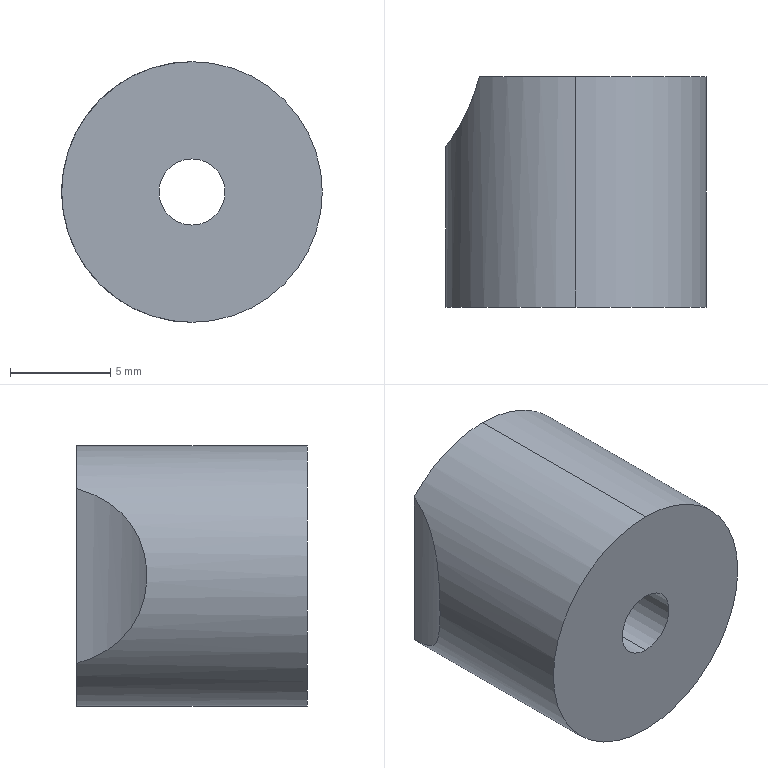Part | STEP file | BU-A15b | 1 solid | 7 faces | box 13 x 11.5 x 13 mm | volume 1411 mm3 | cylinder 5 | plane 2 | commonest cylinder face diameters 3.3 x2 13 x2 20 x1
STEP:
#1=CARTESIAN_POINT('',(0.,0.,0.));
#2=DIRECTION('',(0.,0.,1.));
#3=DIRECTION('',(1.,0.,0.));
#4=AXIS2_PLACEMENT_3D('',#1,#2,#3);
#5=CARTESIAN_POINT('',(0.,11.5,-1.65));
#6=VERTEX_POINT('',#5);
#7=CARTESIAN_POINT('',(0.,0.,-1.65));
#8=VERTEX_POINT('',#7);
#9=CARTESIAN_POINT('',(0.,0.,-1.65));
#10=DIRECTION('',(0.,-1.,0.));
#11=VECTOR('',#10,1.);
#12=LINE('',#9,#11);
#13=CARTESIAN_POINT('',(0.,0.,0.));
#14=DIRECTION('',(0.,-1.,0.));
#15=DIRECTION('',(0.,0.,-1.));
#16=AXIS2_PLACEMENT_3D('',#13,#14,#15);
#17=CYLINDRICAL_SURFACE('',#16,1.65);
#18=CARTESIAN_POINT('',(6.283,0.));
#19=DIRECTION('',(0.,1.));
#20=VECTOR('',#19,1.);
#21=LINE('',#18,#20);
#22=(GEOMETRIC_REPRESENTATION_CONTEXT(2)PARAMETRIC_REPRESENTATION_CONTEXT()REPRESENTATION_CONTEXT('',''));
#23=DEFINITIONAL_REPRESENTATION('',(#21),#22);
#24=PCURVE('',#17,#23);
#25=CARTESIAN_POINT('',(0.,0.,0.));
#26=DIRECTION('',(0.,-1.,0.));
#27=DIRECTION('',(0.,0.,-1.));
#28=AXIS2_PLACEMENT_3D('',#25,#26,#27);
#29=CYLINDRICAL_SURFACE('',#28,1.65);
#30=CARTESIAN_POINT('',(0.,0.));
#31=DIRECTION('',(0.,1.));
#32=VECTOR('',#31,1.);
#33=LINE('',#30,#32);
#34=(GEOMETRIC_REPRESENTATION_CONTEXT(2)PARAMETRIC_REPRESENTATION_CONTEXT()REPRESENTATION_CONTEXT('',''));
#35=DEFINITIONAL_REPRESENTATION('',(#33),#34);
#36=PCURVE('',#29,#35);
#37=SURFACE_CURVE('',#12,(#24,#36),.PCURVE_S1.);
#38=EDGE_CURVE('',#6,#8,#37,.T.);
#39=ORIENTED_EDGE('',*,*,#38,.T.);
#40=CARTESIAN_POINT('',(0.,0.,1.65));
#41=VERTEX_POINT('',#40);
#42=CARTESIAN_POINT('',(0.,0.,0.));
#43=DIRECTION('',(0.,-1.,0.));
#44=DIRECTION('',(0.,0.,-1.));
#45=AXIS2_PLACEMENT_3D('',#42,#43,#44);
#46=CIRCLE('',#45,1.65);
#47=CARTESIAN_POINT('',(0.,0.));
#48=DIRECTION('',(1.,0.));
#49=VECTOR('',#48,1.);
#50=LINE('',#47,#49);
#51=(GEOMETRIC_REPRESENTATION_CONTEXT(2)PARAMETRIC_REPRESENTATION_CONTEXT()REPRESENTATION_CONTEXT('',''));
#52=DEFINITIONAL_REPRESENTATION('',(#50),#51);
#53=PCURVE('',#17,#52);
#54=CARTESIAN_POINT('',(0.,0.,0.));
#55=DIRECTION('',(0.,1.,0.));
#56=DIRECTION('',(0.,0.,1.));
#57=AXIS2_PLACEMENT_3D('',#54,#55,#56);
#58=PLANE('',#57);
#59=CARTESIAN_POINT('',(-1.65,0.));
#60=CARTESIAN_POINT('',(-1.65,2.858));
#61=CARTESIAN_POINT('',(0.825,1.429));
#62=CARTESIAN_POINT('',(3.3,0.));
#63=CARTESIAN_POINT('',(0.825,-1.429));
#64=CARTESIAN_POINT('',(-1.65,-2.858));
#65=CARTESIAN_POINT('',(-1.65,0.));
#66=(BOUNDED_CURVE()B_SPLINE_CURVE(2,(#59,#60,#61,#62,#63,#64,#65),.UNSPECIFIED.,.T.,.F.)B_SPLINE_CURVE_WITH_KNOTS((1,2,2,2,2,1),(-2.094,0.,2.094,4.189,6.283,8.378),.UNSPECIFIED.)CURVE()GEOMETRIC_REPRESENTATION_ITEM()RATIONAL_B_SPLINE_CURVE((1.,0.5,1.,0.5,1.,0.5,1.))REPRESENTATION_ITEM(''));
#67=(GEOMETRIC_REPRESENTATION_CONTEXT(2)PARAMETRIC_REPRESENTATION_CONTEXT()REPRESENTATION_CONTEXT('',''));
#68=DEFINITIONAL_REPRESENTATION('',(#66),#67);
#69=PCURVE('',#58,#68);
#70=SURFACE_CURVE('',#46,(#53,#69),.PCURVE_S1.);
#71=EDGE_CURVE('',#41,#8,#70,.T.);
#72=ORIENTED_EDGE('',*,*,#71,.F.);
#73=CARTESIAN_POINT('',(0.,11.5,1.65));
#74=VERTEX_POINT('',#73);
#75=CARTESIAN_POINT('',(0.,0.,1.65));
#76=DIRECTION('',(0.,-1.,0.));
#77=VECTOR('',#76,1.);
#78=LINE('',#75,#77);
#79=CARTESIAN_POINT('',(3.142,0.));
#80=DIRECTION('',(0.,1.));
#81=VECTOR('',#80,1.);
#82=LINE('',#79,#81);
#83=(GEOMETRIC_REPRESENTATION_CONTEXT(2)PARAMETRIC_REPRESENTATION_CONTEXT()REPRESENTATION_CONTEXT('',''));
#84=DEFINITIONAL_REPRESENTATION('',(#82),#83);
#85=PCURVE('',#17,#84);
#86=CARTESIAN_POINT('',(3.142,0.));
#87=DIRECTION('',(0.,1.));
#88=VECTOR('',#87,1.);
#89=LINE('',#86,#88);
#90=(GEOMETRIC_REPRESENTATION_CONTEXT(2)PARAMETRIC_REPRESENTATION_CONTEXT()REPRESENTATION_CONTEXT('',''));
#91=DEFINITIONAL_REPRESENTATION('',(#89),#90);
#92=PCURVE('',#29,#91);
#93=SURFACE_CURVE('',#78,(#85,#92),.PCURVE_S1.);
#94=EDGE_CURVE('',#74,#41,#93,.T.);
#95=ORIENTED_EDGE('',*,*,#94,.F.);
#96=CARTESIAN_POINT('',(0.,11.5,0.));
#97=DIRECTION('',(0.,-1.,0.));
#98=DIRECTION('',(0.,0.,-1.));
#99=AXIS2_PLACEMENT_3D('',#96,#97,#98);
#100=CIRCLE('',#99,1.65);
#101=CARTESIAN_POINT('',(0.,-11.5));
#102=DIRECTION('',(1.,0.));
#103=VECTOR('',#102,1.);
#104=LINE('',#101,#103);
#105=(GEOMETRIC_REPRESENTATION_CONTEXT(2)PARAMETRIC_REPRESENTATION_CONTEXT()REPRESENTATION_CONTEXT('',''));
#106=DEFINITIONAL_REPRESENTATION('',(#104),#105);
#107=PCURVE('',#17,#106);
#108=CARTESIAN_POINT('',(0.,11.5,0.));
#109=DIRECTION('',(0.,-1.,0.));
#110=DIRECTION('',(0.,0.,-1.));
#111=AXIS2_PLACEMENT_3D('',#108,#109,#110);
#112=PLANE('',#111);
#113=CARTESIAN_POINT('',(0.,0.));
#114=DIRECTION('',(1.,0.));
#115=AXIS2_PLACEMENT_2D('',#113,#114);
#116=CIRCLE('',#115,1.65);
#117=(GEOMETRIC_REPRESENTATION_CONTEXT(2)PARAMETRIC_REPRESENTATION_CONTEXT()REPRESENTATION_CONTEXT('',''));
#118=DEFINITIONAL_REPRESENTATION('',(#116),#117);
#119=PCURVE('',#112,#118);
#120=SURFACE_CURVE('',#100,(#107,#119),.PCURVE_S1.);
#121=EDGE_CURVE('',#74,#6,#120,.T.);
#122=ORIENTED_EDGE('',*,*,#121,.T.);
#123=EDGE_LOOP('',(#39,#72,#95,#122));
#124=FACE_BOUND('',#123,.F.);
#125=ADVANCED_FACE('',(#124),#17,.F.);
#126=CARTESIAN_POINT('',(0.,0.,6.5));
#127=VERTEX_POINT('',#126);
#128=CARTESIAN_POINT('',(0.,0.,-6.5));
#129=VERTEX_POINT('',#128);
#130=CARTESIAN_POINT('',(0.,0.,0.));
#131=DIRECTION('',(0.,1.,0.));
#132=DIRECTION('',(0.,0.,1.));
#133=AXIS2_PLACEMENT_3D('',#130,#131,#132);
#134=CIRCLE('',#133,6.5);
#135=CARTESIAN_POINT('',(0.,0.,0.));
#136=DIRECTION('',(0.,1.,0.));
#137=DIRECTION('',(0.,0.,1.));
#138=AXIS2_PLACEMENT_3D('',#135,#136,#137);
#139=CYLINDRICAL_SURFACE('',#138,6.5);
#140=CARTESIAN_POINT('',(0.,0.));
#141=DIRECTION('',(1.,0.));
#142=VECTOR('',#141,1.);
#143=LINE('',#140,#142);
#144=(GEOMETRIC_REPRESENTATION_CONTEXT(2)PARAMETRIC_REPRESENTATION_CONTEXT()REPRESENTATION_CONTEXT('',''));
#145=DEFINITIONAL_REPRESENTATION('',(#143),#144);
#146=PCURVE('',#139,#145);
#147=CARTESIAN_POINT('',(0.,0.));
#148=DIRECTION('',(1.,0.));
#149=AXIS2_PLACEMENT_2D('',#147,#148);
#150=CIRCLE('',#149,6.5);
#151=(GEOMETRIC_REPRESENTATION_CONTEXT(2)PARAMETRIC_REPRESENTATION_CONTEXT()REPRESENTATION_CONTEXT('',''));
#152=DEFINITIONAL_REPRESENTATION('',(#150),#151);
#153=PCURVE('',#58,#152);
#154=SURFACE_CURVE('',#134,(#146,#153),.PCURVE_S1.);
#155=EDGE_CURVE('',#127,#129,#154,.T.);
#156=ORIENTED_EDGE('',*,*,#155,.T.);
#157=CARTESIAN_POINT('',(0.,11.5,-6.5));
#158=VERTEX_POINT('',#157);
#159=CARTESIAN_POINT('',(0.,0.,-6.5));
#160=DIRECTION('',(0.,1.,0.));
#161=VECTOR('',#160,1.);
#162=LINE('',#159,#161);
#163=CARTESIAN_POINT('',(3.142,0.));
#164=DIRECTION('',(0.,1.));
#165=VECTOR('',#164,1.);
#166=LINE('',#163,#165);
#167=(GEOMETRIC_REPRESENTATION_CONTEXT(2)PARAMETRIC_REPRESENTATION_CONTEXT()REPRESENTATION_CONTEXT('',''));
#168=DEFINITIONAL_REPRESENTATION('',(#166),#167);
#169=PCURVE('',#139,#168);
#170=CARTESIAN_POINT('',(0.,0.,0.));
#171=DIRECTION('',(0.,1.,0.));
#172=DIRECTION('',(0.,0.,1.));
#173=AXIS2_PLACEMENT_3D('',#170,#171,#172);
#174=CYLINDRICAL_SURFACE('',#173,6.5);
#175=CARTESIAN_POINT('',(3.142,0.));
#176=DIRECTION('',(0.,1.));
#177=VECTOR('',#176,1.);
#178=LINE('',#175,#177);
#179=(GEOMETRIC_REPRESENTATION_CONTEXT(2)PARAMETRIC_REPRESENTATION_CONTEXT()REPRESENTATION_CONTEXT('',''));
#180=DEFINITIONAL_REPRESENTATION('',(#178),#179);
#181=PCURVE('',#174,#180);
#182=SURFACE_CURVE('',#162,(#169,#181),.PCURVE_S1.);
#183=EDGE_CURVE('',#129,#158,#182,.T.);
#184=ORIENTED_EDGE('',*,*,#183,.T.);
#185=CARTESIAN_POINT('',(0.,11.5,6.5));
#186=VERTEX_POINT('',#185);
#187=CARTESIAN_POINT('',(0.,11.5,0.));
#188=DIRECTION('',(0.,1.,0.));
#189=DIRECTION('',(0.,0.,1.));
#190=AXIS2_PLACEMENT_3D('',#187,#188,#189);
#191=CIRCLE('',#190,6.5);
#192=CARTESIAN_POINT('',(0.,11.5));
#193=DIRECTION('',(1.,0.));
#194=VECTOR('',#193,1.);
#195=LINE('',#192,#194);
#196=(GEOMETRIC_REPRESENTATION_CONTEXT(2)PARAMETRIC_REPRESENTATION_CONTEXT()REPRESENTATION_CONTEXT('',''));
#197=DEFINITIONAL_REPRESENTATION('',(#195),#196);
#198=PCURVE('',#139,#197);
#199=CARTESIAN_POINT('',(-6.5,0.));
#200=CARTESIAN_POINT('',(-6.5,11.258));
#201=CARTESIAN_POINT('',(3.25,5.629));
#202=CARTESIAN_POINT('',(13.,0.));
#203=CARTESIAN_POINT('',(3.25,-5.629));
#204=CARTESIAN_POINT('',(-6.5,-11.258));
#205=CARTESIAN_POINT('',(-6.5,0.));
#206=(BOUNDED_CURVE()B_SPLINE_CURVE(2,(#199,#200,#201,#202,#203,#204,#205),.UNSPECIFIED.,.T.,.F.)B_SPLINE_CURVE_WITH_KNOTS((1,2,2,2,2,1),(-2.094,0.,2.094,4.189,6.283,8.378),.UNSPECIFIED.)CURVE()GEOMETRIC_REPRESENTATION_ITEM()RATIONAL_B_SPLINE_CURVE((1.,0.5,1.,0.5,1.,0.5,1.))REPRESENTATION_ITEM(''));
#207=(GEOMETRIC_REPRESENTATION_CONTEXT(2)PARAMETRIC_REPRESENTATION_CONTEXT()REPRESENTATION_CONTEXT('',''));
#208=DEFINITIONAL_REPRESENTATION('',(#206),#207);
#209=PCURVE('',#112,#208);
#210=SURFACE_CURVE('',#191,(#198,#209),.PCURVE_S1.);
#211=EDGE_CURVE('',#186,#158,#210,.T.);
#212=ORIENTED_EDGE('',*,*,#211,.F.);
#213=CARTESIAN_POINT('',(0.,0.,6.5));
#214=DIRECTION('',(0.,1.,0.));
#215=VECTOR('',#214,1.);
#216=LINE('',#213,#215);
#217=CARTESIAN_POINT('',(0.,0.));
#218=DIRECTION('',(0.,1.));
#219=VECTOR('',#218,1.);
#220=LINE('',#217,#219);
#221=(GEOMETRIC_REPRESENTATION_CONTEXT(2)PARAMETRIC_REPRESENTATION_CONTEXT()REPRESENTATION_CONTEXT('',''));
#222=DEFINITIONAL_REPRESENTATION('',(#220),#221);
#223=PCURVE('',#139,#222);
#224=CARTESIAN_POINT('',(6.283,0.));
#225=DIRECTION('',(0.,1.));
#226=VECTOR('',#225,1.);
#227=LINE('',#224,#226);
#228=(GEOMETRIC_REPRESENTATION_CONTEXT(2)PARAMETRIC_REPRESENTATION_CONTEXT()REPRESENTATION_CONTEXT('',''));
#229=DEFINITIONAL_REPRESENTATION('',(#227),#228);
#230=PCURVE('',#174,#229);
#231=SURFACE_CURVE('',#216,(#223,#230),.PCURVE_S1.);
#232=EDGE_CURVE('',#127,#186,#231,.T.);
#233=ORIENTED_EDGE('',*,*,#232,.F.);
#234=EDGE_LOOP('',(#156,#184,#212,#233));
#235=FACE_BOUND('',#234,.T.);
#236=ADVANCED_FACE('',(#235),#139,.T.);
#237=CARTESIAN_POINT('',(0.,11.5,0.));
#238=DIRECTION('',(0.,-1.,0.));
#239=DIRECTION('',(0.,0.,-1.));
#240=AXIS2_PLACEMENT_3D('',#237,#238,#239);
#241=CIRCLE('',#240,1.65);
#242=CARTESIAN_POINT('',(0.,0.));
#243=DIRECTION('',(1.,0.));
#244=AXIS2_PLACEMENT_2D('',#242,#243);
#245=CIRCLE('',#244,1.65);
#246=(GEOMETRIC_REPRESENTATION_CONTEXT(2)PARAMETRIC_REPRESENTATION_CONTEXT()REPRESENTATION_CONTEXT('',''));
#247=DEFINITIONAL_REPRESENTATION('',(#245),#246);
#248=PCURVE('',#112,#247);
#249=CARTESIAN_POINT('',(0.,-11.5));
#250=DIRECTION('',(1.,0.));
#251=VECTOR('',#250,1.);
#252=LINE('',#249,#251);
#253=(GEOMETRIC_REPRESENTATION_CONTEXT(2)PARAMETRIC_REPRESENTATION_CONTEXT()REPRESENTATION_CONTEXT('',''));
#254=DEFINITIONAL_REPRESENTATION('',(#252),#253);
#255=PCURVE('',#29,#254);
#256=SURFACE_CURVE('',#241,(#248,#255),.PCURVE_S1.);
#257=EDGE_CURVE('',#6,#74,#256,.T.);
#258=ORIENTED_EDGE('',*,*,#257,.T.);
#259=ORIENTED_EDGE('',*,*,#121,.T.);
#260=EDGE_LOOP('',(#258,#259));
#261=FACE_BOUND('',#260,.T.);
#262=CARTESIAN_POINT('',(-4.818,11.5,4.364));
#263=VERTEX_POINT('',#262);
#264=CARTESIAN_POINT('',(0.,11.5,0.));
#265=DIRECTION('',(0.,1.,0.));
#266=DIRECTION('',(0.,0.,1.));
#267=AXIS2_PLACEMENT_3D('',#264,#265,#266);
#268=CIRCLE('',#267,6.5);
#269=CARTESIAN_POINT('',(-6.5,0.));
#270=CARTESIAN_POINT('',(-6.5,11.258));
#271=CARTESIAN_POINT('',(3.25,5.629));
#272=CARTESIAN_POINT('',(13.,0.));
#273=CARTESIAN_POINT('',(3.25,-5.629));
#274=CARTESIAN_POINT('',(-6.5,-11.258));
#275=CARTESIAN_POINT('',(-6.5,0.));
#276=(BOUNDED_CURVE()B_SPLINE_CURVE(2,(#269,#270,#271,#272,#273,#274,#275),.UNSPECIFIED.,.T.,.F.)B_SPLINE_CURVE_WITH_KNOTS((1,2,2,2,2,1),(-2.094,0.,2.094,4.189,6.283,8.378),.UNSPECIFIED.)CURVE()GEOMETRIC_REPRESENTATION_ITEM()RATIONAL_B_SPLINE_CURVE((1.,0.5,1.,0.5,1.,0.5,1.))REPRESENTATION_ITEM(''));
#277=(GEOMETRIC_REPRESENTATION_CONTEXT(2)PARAMETRIC_REPRESENTATION_CONTEXT()REPRESENTATION_CONTEXT('',''));
#278=DEFINITIONAL_REPRESENTATION('',(#276),#277);
#279=PCURVE('',#112,#278);
#280=CARTESIAN_POINT('',(0.,11.5));
#281=DIRECTION('',(1.,0.));
#282=VECTOR('',#281,1.);
#283=LINE('',#280,#282);
#284=(GEOMETRIC_REPRESENTATION_CONTEXT(2)PARAMETRIC_REPRESENTATION_CONTEXT()REPRESENTATION_CONTEXT('',''));
#285=DEFINITIONAL_REPRESENTATION('',(#283),#284);
#286=PCURVE('',#174,#285);
#287=SURFACE_CURVE('',#268,(#279,#286),.PCURVE_S1.);
#288=EDGE_CURVE('',#263,#186,#287,.T.);
#289=ORIENTED_EDGE('',*,*,#288,.T.);
#290=ORIENTED_EDGE('',*,*,#211,.T.);
#291=CARTESIAN_POINT('',(-4.818,11.5,-4.364));
#292=VERTEX_POINT('',#291);
#293=CARTESIAN_POINT('',(0.,11.5,0.));
#294=DIRECTION('',(0.,1.,0.));
#295=DIRECTION('',(0.,0.,1.));
#296=AXIS2_PLACEMENT_3D('',#293,#294,#295);
#297=CIRCLE('',#296,6.5);
#298=CARTESIAN_POINT('',(-6.5,0.));
#299=CARTESIAN_POINT('',(-6.5,11.258));
#300=CARTESIAN_POINT('',(3.25,5.629));
#301=CARTESIAN_POINT('',(13.,0.));
#302=CARTESIAN_POINT('',(3.25,-5.629));
#303=CARTESIAN_POINT('',(-6.5,-11.258));
#304=CARTESIAN_POINT('',(-6.5,0.));
#305=(BOUNDED_CURVE()B_SPLINE_CURVE(2,(#298,#299,#300,#301,#302,#303,#304),.UNSPECIFIED.,.T.,.F.)B_SPLINE_CURVE_WITH_KNOTS((1,2,2,2,2,1),(-2.094,0.,2.094,4.189,6.283,8.378),.UNSPECIFIED.)CURVE()GEOMETRIC_REPRESENTATION_ITEM()RATIONAL_B_SPLINE_CURVE((1.,0.5,1.,0.5,1.,0.5,1.))REPRESENTATION_ITEM(''));
#306=(GEOMETRIC_REPRESENTATION_CONTEXT(2)PARAMETRIC_REPRESENTATION_CONTEXT()REPRESENTATION_CONTEXT('',''));
#307=DEFINITIONAL_REPRESENTATION('',(#305),#306);
#308=PCURVE('',#112,#307);
#309=CARTESIAN_POINT('',(0.,11.5));
#310=DIRECTION('',(1.,0.));
#311=VECTOR('',#310,1.);
#312=LINE('',#309,#311);
#313=(GEOMETRIC_REPRESENTATION_CONTEXT(2)PARAMETRIC_REPRESENTATION_CONTEXT()REPRESENTATION_CONTEXT('',''));
#314=DEFINITIONAL_REPRESENTATION('',(#312),#313);
#315=PCURVE('',#174,#314);
#316=SURFACE_CURVE('',#297,(#308,#315),.PCURVE_S1.);
#317=EDGE_CURVE('',#158,#292,#316,.T.);
#318=ORIENTED_EDGE('',*,*,#317,.T.);
#319=CARTESIAN_POINT('',(-4.818,11.5,-6.5));
#320=DIRECTION('',(0.,0.,1.));
#321=VECTOR('',#320,1.);
#322=LINE('',#319,#321);
#323=CARTESIAN_POINT('',(6.5,-4.818));
#324=DIRECTION('',(-1.,0.));
#325=VECTOR('',#324,1.);
#326=LINE('',#323,#325);
#327=(GEOMETRIC_REPRESENTATION_CONTEXT(2)PARAMETRIC_REPRESENTATION_CONTEXT()REPRESENTATION_CONTEXT('',''));
#328=DEFINITIONAL_REPRESENTATION('',(#326),#327);
#329=PCURVE('',#112,#328);
#330=CARTESIAN_POINT('',(-14.5,14.,-6.5));
#331=DIRECTION('',(0.,0.,1.));
#332=DIRECTION('',(1.,0.,0.));
#333=AXIS2_PLACEMENT_3D('',#330,#331,#332);
#334=CYLINDRICAL_SURFACE('',#333,10.);
#335=CARTESIAN_POINT('',(6.031,0.));
#336=DIRECTION('',(0.,1.));
#337=VECTOR('',#336,1.);
#338=LINE('',#335,#337);
#339=(GEOMETRIC_REPRESENTATION_CONTEXT(2)PARAMETRIC_REPRESENTATION_CONTEXT()REPRESENTATION_CONTEXT('',''));
#340=DEFINITIONAL_REPRESENTATION('',(#338),#339);
#341=PCURVE('',#334,#340);
#342=SURFACE_CURVE('',#322,(#329,#341),.PCURVE_S1.);
#343=EDGE_CURVE('',#292,#263,#342,.T.);
#344=ORIENTED_EDGE('',*,*,#343,.T.);
#345=EDGE_LOOP('',(#289,#290,#318,#344));
#346=FACE_BOUND('',#345,.T.);
#347=ADVANCED_FACE('',(#261,#346),#112,.F.);
#348=ORIENTED_EDGE('',*,*,#183,.F.);
#349=CARTESIAN_POINT('',(0.,0.,0.));
#350=DIRECTION('',(0.,1.,0.));
#351=DIRECTION('',(0.,0.,1.));
#352=AXIS2_PLACEMENT_3D('',#349,#350,#351);
#353=CIRCLE('',#352,6.5);
#354=CARTESIAN_POINT('',(0.,0.));
#355=DIRECTION('',(1.,0.));
#356=VECTOR('',#355,1.);
#357=LINE('',#354,#356);
#358=(GEOMETRIC_REPRESENTATION_CONTEXT(2)PARAMETRIC_REPRESENTATION_CONTEXT()REPRESENTATION_CONTEXT('',''));
#359=DEFINITIONAL_REPRESENTATION('',(#357),#358);
#360=PCURVE('',#174,#359);
#361=CARTESIAN_POINT('',(0.,0.));
#362=DIRECTION('',(1.,0.));
#363=AXIS2_PLACEMENT_2D('',#361,#362);
#364=CIRCLE('',#363,6.5);
#365=(GEOMETRIC_REPRESENTATION_CONTEXT(2)PARAMETRIC_REPRESENTATION_CONTEXT()REPRESENTATION_CONTEXT('',''));
#366=DEFINITIONAL_REPRESENTATION('',(#364),#365);
#367=PCURVE('',#58,#366);
#368=SURFACE_CURVE('',#353,(#360,#367),.PCURVE_S1.);
#369=EDGE_CURVE('',#129,#127,#368,.T.);
#370=ORIENTED_EDGE('',*,*,#369,.T.);
#371=ORIENTED_EDGE('',*,*,#232,.T.);
#372=ORIENTED_EDGE('',*,*,#288,.F.);
#373=CARTESIAN_POINT('',(-4.818,11.5,4.364));
#374=CARTESIAN_POINT('',(-4.945,11.006,4.223));
#375=CARTESIAN_POINT('',(-5.105,10.544,4.036));
#376=CARTESIAN_POINT('',(-5.374,9.904,3.659));
#377=CARTESIAN_POINT('',(-5.469,9.7,3.517));
#378=CARTESIAN_POINT('',(-5.657,9.325,3.206));
#379=CARTESIAN_POINT('',(-5.752,9.152,3.035));
#380=CARTESIAN_POINT('',(-5.934,8.837,2.66));
#381=CARTESIAN_POINT('',(-6.024,8.692,2.454));
#382=CARTESIAN_POINT('',(-6.183,8.446,2.018));
#383=CARTESIAN_POINT('',(-6.254,8.342,1.789));
#384=CARTESIAN_POINT('',(-6.372,8.174,1.309));
#385=CARTESIAN_POINT('',(-6.419,8.109,1.054));
#386=CARTESIAN_POINT('',(-6.483,8.023,0.5378));
#387=CARTESIAN_POINT('',(-6.499,8.001,0.2774));
#388=CARTESIAN_POINT('',(-6.501,7.999,-0.2484));
#389=CARTESIAN_POINT('',(-6.485,8.02,-0.5153));
#390=CARTESIAN_POINT('',(-6.423,8.104,-1.03));
#391=CARTESIAN_POINT('',(-6.377,8.166,-1.281));
#392=CARTESIAN_POINT('',(-6.259,8.334,-1.77));
#393=CARTESIAN_POINT('',(-6.188,8.438,-2.003));
#394=CARTESIAN_POINT('',(-6.029,8.683,-2.439));
#395=CARTESIAN_POINT('',(-5.941,8.825,-2.646));
#396=CARTESIAN_POINT('',(-5.757,9.143,-3.026));
#397=CARTESIAN_POINT('',(-5.662,9.317,-3.198));
#398=CARTESIAN_POINT('',(-5.472,9.694,-3.513));
#399=CARTESIAN_POINT('',(-5.377,9.898,-3.655));
#400=CARTESIAN_POINT('',(-5.107,10.538,-4.033));
#401=CARTESIAN_POINT('',(-4.945,11.005,-4.223));
#402=CARTESIAN_POINT('',(-4.818,11.5,-4.364));
#403=B_SPLINE_CURVE_WITH_KNOTS('',3,(#373,#374,#375,#376,#377,#378,#379,#380,#381,#382,#383,#384,#385,#386,#387,#388,#389,#390,#391,#392,#393,#394,#395,#396,#397,#398,#399,#400,#401,#402),.UNSPECIFIED.,.F.,.F.,(4,2,2,2,2,2,2,2,2,2,2,2,2,2,4),(0.,0.00157,0.002355,0.00314,0.003925,0.004709,0.005494,0.006279,0.007064,0.007849,0.008634,0.009419,0.0102,0.01099,0.01256),.UNSPECIFIED.);
#404=CARTESIAN_POINT('',(5.448,11.5));
#405=CARTESIAN_POINT('',(5.445,11.44));
#406=CARTESIAN_POINT('',(5.438,11.321));
#407=CARTESIAN_POINT('',(5.426,11.146));
#408=CARTESIAN_POINT('',(5.413,10.974));
#409=CARTESIAN_POINT('',(5.4,10.804));
#410=CARTESIAN_POINT('',(5.386,10.637));
#411=CARTESIAN_POINT('',(5.371,10.474));
#412=CARTESIAN_POINT('',(5.355,10.313));
#413=CARTESIAN_POINT('',(5.338,10.156));
#414=CARTESIAN_POINT('',(5.321,10.001));
#415=CARTESIAN_POINT('',(5.302,9.851));
#416=CARTESIAN_POINT('',(5.283,9.704));
#417=CARTESIAN_POINT('',(5.264,9.563));
#418=CARTESIAN_POINT('',(5.243,9.428));
#419=CARTESIAN_POINT('',(5.222,9.297));
#420=CARTESIAN_POINT('',(5.2,9.172));
#421=CARTESIAN_POINT('',(5.178,9.052));
#422=CARTESIAN_POINT('',(5.154,8.937));
#423=CARTESIAN_POINT('',(5.13,8.827));
#424=CARTESIAN_POINT('',(5.105,8.723));
#425=CARTESIAN_POINT('',(5.08,8.625));
#426=CARTESIAN_POINT('',(5.054,8.535));
#427=CARTESIAN_POINT('',(5.028,8.451));
#428=CARTESIAN_POINT('',(5.001,8.374));
#429=CARTESIAN_POINT('',(4.974,8.305));
#430=CARTESIAN_POINT('',(4.946,8.242));
#431=CARTESIAN_POINT('',(4.918,8.186));
#432=CARTESIAN_POINT('',(4.889,8.137));
#433=CARTESIAN_POINT('',(4.861,8.095));
#434=CARTESIAN_POINT('',(4.831,8.061));
#435=CARTESIAN_POINT('',(4.802,8.034));
#436=CARTESIAN_POINT('',(4.773,8.015));
#437=CARTESIAN_POINT('',(4.744,8.003));
#438=CARTESIAN_POINT('',(4.715,7.999));
#439=CARTESIAN_POINT('',(4.685,8.002));
#440=CARTESIAN_POINT('',(4.656,8.013));
#441=CARTESIAN_POINT('',(4.626,8.031));
#442=CARTESIAN_POINT('',(4.597,8.057));
#443=CARTESIAN_POINT('',(4.568,8.09));
#444=CARTESIAN_POINT('',(4.539,8.131));
#445=CARTESIAN_POINT('',(4.511,8.178));
#446=CARTESIAN_POINT('',(4.482,8.234));
#447=CARTESIAN_POINT('',(4.454,8.297));
#448=CARTESIAN_POINT('',(4.427,8.367));
#449=CARTESIAN_POINT('',(4.4,8.443));
#450=CARTESIAN_POINT('',(4.373,8.527));
#451=CARTESIAN_POINT('',(4.347,8.616));
#452=CARTESIAN_POINT('',(4.322,8.713));
#453=CARTESIAN_POINT('',(4.297,8.817));
#454=CARTESIAN_POINT('',(4.273,8.926));
#455=CARTESIAN_POINT('',(4.249,9.042));
#456=CARTESIAN_POINT('',(4.226,9.163));
#457=CARTESIAN_POINT('',(4.204,9.289));
#458=CARTESIAN_POINT('',(4.183,9.42));
#459=CARTESIAN_POINT('',(4.162,9.557));
#460=CARTESIAN_POINT('',(4.142,9.698));
#461=CARTESIAN_POINT('',(4.123,9.845));
#462=CARTESIAN_POINT('',(4.105,9.996));
#463=CARTESIAN_POINT('',(4.087,10.15));
#464=CARTESIAN_POINT('',(4.07,10.308));
#465=CARTESIAN_POINT('',(4.055,10.469));
#466=CARTESIAN_POINT('',(4.039,10.633));
#467=CARTESIAN_POINT('',(4.025,10.801));
#468=CARTESIAN_POINT('',(4.012,10.971));
#469=CARTESIAN_POINT('',(3.999,11.145));
#470=CARTESIAN_POINT('',(3.987,11.321));
#471=CARTESIAN_POINT('',(3.98,11.44));
#472=CARTESIAN_POINT('',(3.976,11.5));
#473=B_SPLINE_CURVE_WITH_KNOTS('',3,(#404,#405,#406,#407,#408,#409,#410,#411,#412,#413,#414,#415,#416,#417,#418,#419,#420,#421,#422,#423,#424,#425,#426,#427,#428,#429,#430,#431,#432,#433,#434,#435,#436,#437,#438,#439,#440,#441,#442,#443,#444,#445,#446,#447,#448,#449,#450,#451,#452,#453,#454,#455,#456,#457,#458,#459,#460,#461,#462,#463,#464,#465,#466,#467,#468,#469,#470,#471,#472),.UNSPECIFIED.,.F.,.F.,(4,1,1,1,1,1,1,1,1,1,1,1,1,1,1,1,1,1,1,1,1,1,1,1,1,1,1,1,1,1,1,1,1,1,1,1,1,1,1,1,1,1,1,1,1,1,1,1,1,1,1,1,1,1,1,1,1,1,1,1,1,1,1,1,1,1,4),(0.,0.0001903,0.0003806,0.0005708,0.0007611,0.0009514,0.001142,0.001332,0.001522,0.001713,0.001903,0.002093,0.002283,0.002474,0.002664,0.002854,0.003044,0.003235,0.003425,0.003615,0.003806,0.003996,0.004186,0.004376,0.004567,0.004757,0.004947,0.005138,0.005328,0.005518,0.005708,0.005899,0.006089,0.006279,0.006469,0.00666,0.00685,0.00704,0.007231,0.007421,0.007611,0.007801,0.007992,0.008182,0.008372,0.008563,0.008753,0.008943,0.009133,0.009324,0.009514,0.009704,0.009895,0.01008,0.01028,0.01047,0.01066,0.01085,0.01104,0.01123,0.01142,0.01161,0.0118,0.01199,0.01218,0.01237,0.01256),.QUASI_UNIFORM_KNOTS.);
#474=(GEOMETRIC_REPRESENTATION_CONTEXT(2)PARAMETRIC_REPRESENTATION_CONTEXT()REPRESENTATION_CONTEXT('',''));
#475=DEFINITIONAL_REPRESENTATION('',(#473),#474);
#476=PCURVE('',#174,#475);
#477=CARTESIAN_POINT('',(6.031,10.864));
#478=CARTESIAN_POINT('',(6.024,10.847));
#479=CARTESIAN_POINT('',(6.012,10.811));
#480=CARTESIAN_POINT('',(5.994,10.754));
#481=CARTESIAN_POINT('',(5.976,10.692));
#482=CARTESIAN_POINT('',(5.958,10.625));
#483=CARTESIAN_POINT('',(5.94,10.554));
#484=CARTESIAN_POINT('',(5.923,10.477));
#485=CARTESIAN_POINT('',(5.906,10.395));
#486=CARTESIAN_POINT('',(5.889,10.308));
#487=CARTESIAN_POINT('',(5.872,10.215));
#488=CARTESIAN_POINT('',(5.855,10.117));
#489=CARTESIAN_POINT('',(5.839,10.013));
#490=CARTESIAN_POINT('',(5.824,9.904));
#491=CARTESIAN_POINT('',(5.808,9.79));
#492=CARTESIAN_POINT('',(5.794,9.671));
#493=CARTESIAN_POINT('',(5.779,9.547));
#494=CARTESIAN_POINT('',(5.766,9.416));
#495=CARTESIAN_POINT('',(5.752,9.28));
#496=CARTESIAN_POINT('',(5.74,9.137));
#497=CARTESIAN_POINT('',(5.727,8.988));
#498=CARTESIAN_POINT('',(5.716,8.835));
#499=CARTESIAN_POINT('',(5.705,8.677));
#500=CARTESIAN_POINT('',(5.695,8.515));
#501=CARTESIAN_POINT('',(5.686,8.349));
#502=CARTESIAN_POINT('',(5.677,8.18));
#503=CARTESIAN_POINT('',(5.67,8.006));
#504=CARTESIAN_POINT('',(5.663,7.827));
#505=CARTESIAN_POINT('',(5.657,7.645));
#506=CARTESIAN_POINT('',(5.651,7.46));
#507=CARTESIAN_POINT('',(5.647,7.272));
#508=CARTESIAN_POINT('',(5.644,7.084));
#509=CARTESIAN_POINT('',(5.642,6.895));
#510=CARTESIAN_POINT('',(5.64,6.705));
#511=CARTESIAN_POINT('',(5.64,6.515));
#512=CARTESIAN_POINT('',(5.64,6.323));
#513=CARTESIAN_POINT('',(5.641,6.131));
#514=CARTESIAN_POINT('',(5.644,5.939));
#515=CARTESIAN_POINT('',(5.647,5.75));
#516=CARTESIAN_POINT('',(5.651,5.564));
#517=CARTESIAN_POINT('',(5.656,5.38));
#518=CARTESIAN_POINT('',(5.662,5.198));
#519=CARTESIAN_POINT('',(5.669,5.019));
#520=CARTESIAN_POINT('',(5.676,4.842));
#521=CARTESIAN_POINT('',(5.685,4.669));
#522=CARTESIAN_POINT('',(5.694,4.501));
#523=CARTESIAN_POINT('',(5.704,4.338));
#524=CARTESIAN_POINT('',(5.715,4.18));
#525=CARTESIAN_POINT('',(5.726,4.026));
#526=CARTESIAN_POINT('',(5.738,3.877));
#527=CARTESIAN_POINT('',(5.751,3.733));
#528=CARTESIAN_POINT('',(5.764,3.595));
#529=CARTESIAN_POINT('',(5.778,3.463));
#530=CARTESIAN_POINT('',(5.793,3.337));
#531=CARTESIAN_POINT('',(5.807,3.216));
#532=CARTESIAN_POINT('',(5.823,3.101));
#533=CARTESIAN_POINT('',(5.839,2.991));
#534=CARTESIAN_POINT('',(5.855,2.887));
#535=CARTESIAN_POINT('',(5.871,2.788));
#536=CARTESIAN_POINT('',(5.888,2.695));
#537=CARTESIAN_POINT('',(5.905,2.608));
#538=CARTESIAN_POINT('',(5.922,2.525));
#539=CARTESIAN_POINT('',(5.94,2.448));
#540=CARTESIAN_POINT('',(5.958,2.376));
#541=CARTESIAN_POINT('',(5.976,2.309));
#542=CARTESIAN_POINT('',(5.994,2.247));
#543=CARTESIAN_POINT('',(6.012,2.189));
#544=CARTESIAN_POINT('',(6.024,2.153));
#545=CARTESIAN_POINT('',(6.031,2.136));
#546=B_SPLINE_CURVE_WITH_KNOTS('',3,(#477,#478,#479,#480,#481,#482,#483,#484,#485,#486,#487,#488,#489,#490,#491,#492,#493,#494,#495,#496,#497,#498,#499,#500,#501,#502,#503,#504,#505,#506,#507,#508,#509,#510,#511,#512,#513,#514,#515,#516,#517,#518,#519,#520,#521,#522,#523,#524,#525,#526,#527,#528,#529,#530,#531,#532,#533,#534,#535,#536,#537,#538,#539,#540,#541,#542,#543,#544,#545),.UNSPECIFIED.,.F.,.F.,(4,1,1,1,1,1,1,1,1,1,1,1,1,1,1,1,1,1,1,1,1,1,1,1,1,1,1,1,1,1,1,1,1,1,1,1,1,1,1,1,1,1,1,1,1,1,1,1,1,1,1,1,1,1,1,1,1,1,1,1,1,1,1,1,1,1,4),(0.,0.0001903,0.0003806,0.0005708,0.0007611,0.0009514,0.001142,0.001332,0.001522,0.001713,0.001903,0.002093,0.002283,0.002474,0.002664,0.002854,0.003044,0.003235,0.003425,0.003615,0.003806,0.003996,0.004186,0.004376,0.004567,0.004757,0.004947,0.005138,0.005328,0.005518,0.005708,0.005899,0.006089,0.006279,0.006469,0.00666,0.00685,0.00704,0.007231,0.007421,0.007611,0.007801,0.007992,0.008182,0.008372,0.008563,0.008753,0.008943,0.009133,0.009324,0.009514,0.009704,0.009895,0.01008,0.01028,0.01047,0.01066,0.01085,0.01104,0.01123,0.01142,0.01161,0.0118,0.01199,0.01218,0.01237,0.01256),.QUASI_UNIFORM_KNOTS.);
#547=(GEOMETRIC_REPRESENTATION_CONTEXT(2)PARAMETRIC_REPRESENTATION_CONTEXT()REPRESENTATION_CONTEXT('',''));
#548=DEFINITIONAL_REPRESENTATION('',(#546),#547);
#549=PCURVE('',#334,#548);
#550=SURFACE_CURVE('',#403,(#476,#549),.PCURVE_S1.);
#551=EDGE_CURVE('',#263,#292,#550,.T.);
#552=ORIENTED_EDGE('',*,*,#551,.T.);
#553=ORIENTED_EDGE('',*,*,#317,.F.);
#554=EDGE_LOOP('',(#348,#370,#371,#372,#552,#553));
#555=FACE_BOUND('',#554,.T.);
#556=ADVANCED_FACE('',(#555),#174,.T.);
#557=CARTESIAN_POINT('',(0.,0.,0.));
#558=DIRECTION('',(0.,-1.,0.));
#559=DIRECTION('',(0.,0.,-1.));
#560=AXIS2_PLACEMENT_3D('',#557,#558,#559);
#561=CIRCLE('',#560,1.65);
#562=CARTESIAN_POINT('',(-1.65,0.));
#563=CARTESIAN_POINT('',(-1.65,2.858));
#564=CARTESIAN_POINT('',(0.825,1.429));
#565=CARTESIAN_POINT('',(3.3,0.));
#566=CARTESIAN_POINT('',(0.825,-1.429));
#567=CARTESIAN_POINT('',(-1.65,-2.858));
#568=CARTESIAN_POINT('',(-1.65,0.));
#569=(BOUNDED_CURVE()B_SPLINE_CURVE(2,(#562,#563,#564,#565,#566,#567,#568),.UNSPECIFIED.,.T.,.F.)B_SPLINE_CURVE_WITH_KNOTS((1,2,2,2,2,1),(-2.094,0.,2.094,4.189,6.283,8.378),.UNSPECIFIED.)CURVE()GEOMETRIC_REPRESENTATION_ITEM()RATIONAL_B_SPLINE_CURVE((1.,0.5,1.,0.5,1.,0.5,1.))REPRESENTATION_ITEM(''));
#570=(GEOMETRIC_REPRESENTATION_CONTEXT(2)PARAMETRIC_REPRESENTATION_CONTEXT()REPRESENTATION_CONTEXT('',''));
#571=DEFINITIONAL_REPRESENTATION('',(#569),#570);
#572=PCURVE('',#58,#571);
#573=CARTESIAN_POINT('',(0.,0.));
#574=DIRECTION('',(1.,0.));
#575=VECTOR('',#574,1.);
#576=LINE('',#573,#575);
#577=(GEOMETRIC_REPRESENTATION_CONTEXT(2)PARAMETRIC_REPRESENTATION_CONTEXT()REPRESENTATION_CONTEXT('',''));
#578=DEFINITIONAL_REPRESENTATION('',(#576),#577);
#579=PCURVE('',#29,#578);
#580=SURFACE_CURVE('',#561,(#572,#579),.PCURVE_S1.);
#581=EDGE_CURVE('',#8,#41,#580,.T.);
#582=ORIENTED_EDGE('',*,*,#581,.F.);
#583=ORIENTED_EDGE('',*,*,#71,.F.);
#584=EDGE_LOOP('',(#582,#583));
#585=FACE_BOUND('',#584,.T.);
#586=ORIENTED_EDGE('',*,*,#155,.F.);
#587=ORIENTED_EDGE('',*,*,#369,.F.);
#588=EDGE_LOOP('',(#586,#587));
#589=FACE_BOUND('',#588,.T.);
#590=ADVANCED_FACE('',(#585,#589),#58,.F.);
#591=ORIENTED_EDGE('',*,*,#551,.T.);
#592=ORIENTED_EDGE('',*,*,#343,.T.);
#593=EDGE_LOOP('',(#591,#592));
#594=FACE_BOUND('',#593,.F.);
#595=ADVANCED_FACE('',(#594),#334,.F.);
#596=ORIENTED_EDGE('',*,*,#581,.F.);
#597=ORIENTED_EDGE('',*,*,#38,.F.);
#598=ORIENTED_EDGE('',*,*,#257,.T.);
#599=ORIENTED_EDGE('',*,*,#94,.T.);
#600=EDGE_LOOP('',(#596,#597,#598,#599));
#601=FACE_BOUND('',#600,.F.);
#602=ADVANCED_FACE('',(#601),#29,.F.);
#603=CLOSED_SHELL('',(#125,#236,#347,#556,#590,#595,#602));
#604=MANIFOLD_SOLID_BREP('',#603);
#605=(LENGTH_UNIT()NAMED_UNIT(*)SI_UNIT(.MILLI.,.METRE.));
#606=UNCERTAINTY_MEASURE_WITH_UNIT(LENGTH_MEASURE(0.00002),#605,'','');
#607=(NAMED_UNIT(*)PLANE_ANGLE_UNIT()SI_UNIT($,.RADIAN.));
#608=(NAMED_UNIT(*)SI_UNIT($,.STERADIAN.)SOLID_ANGLE_UNIT());
#609=(GEOMETRIC_REPRESENTATION_CONTEXT(3)GLOBAL_UNCERTAINTY_ASSIGNED_CONTEXT((#606))GLOBAL_UNIT_ASSIGNED_CONTEXT((#605,#607,#608))REPRESENTATION_CONTEXT('',''));
#610=ADVANCED_BREP_SHAPE_REPRESENTATION('',(#4,#604),#609);